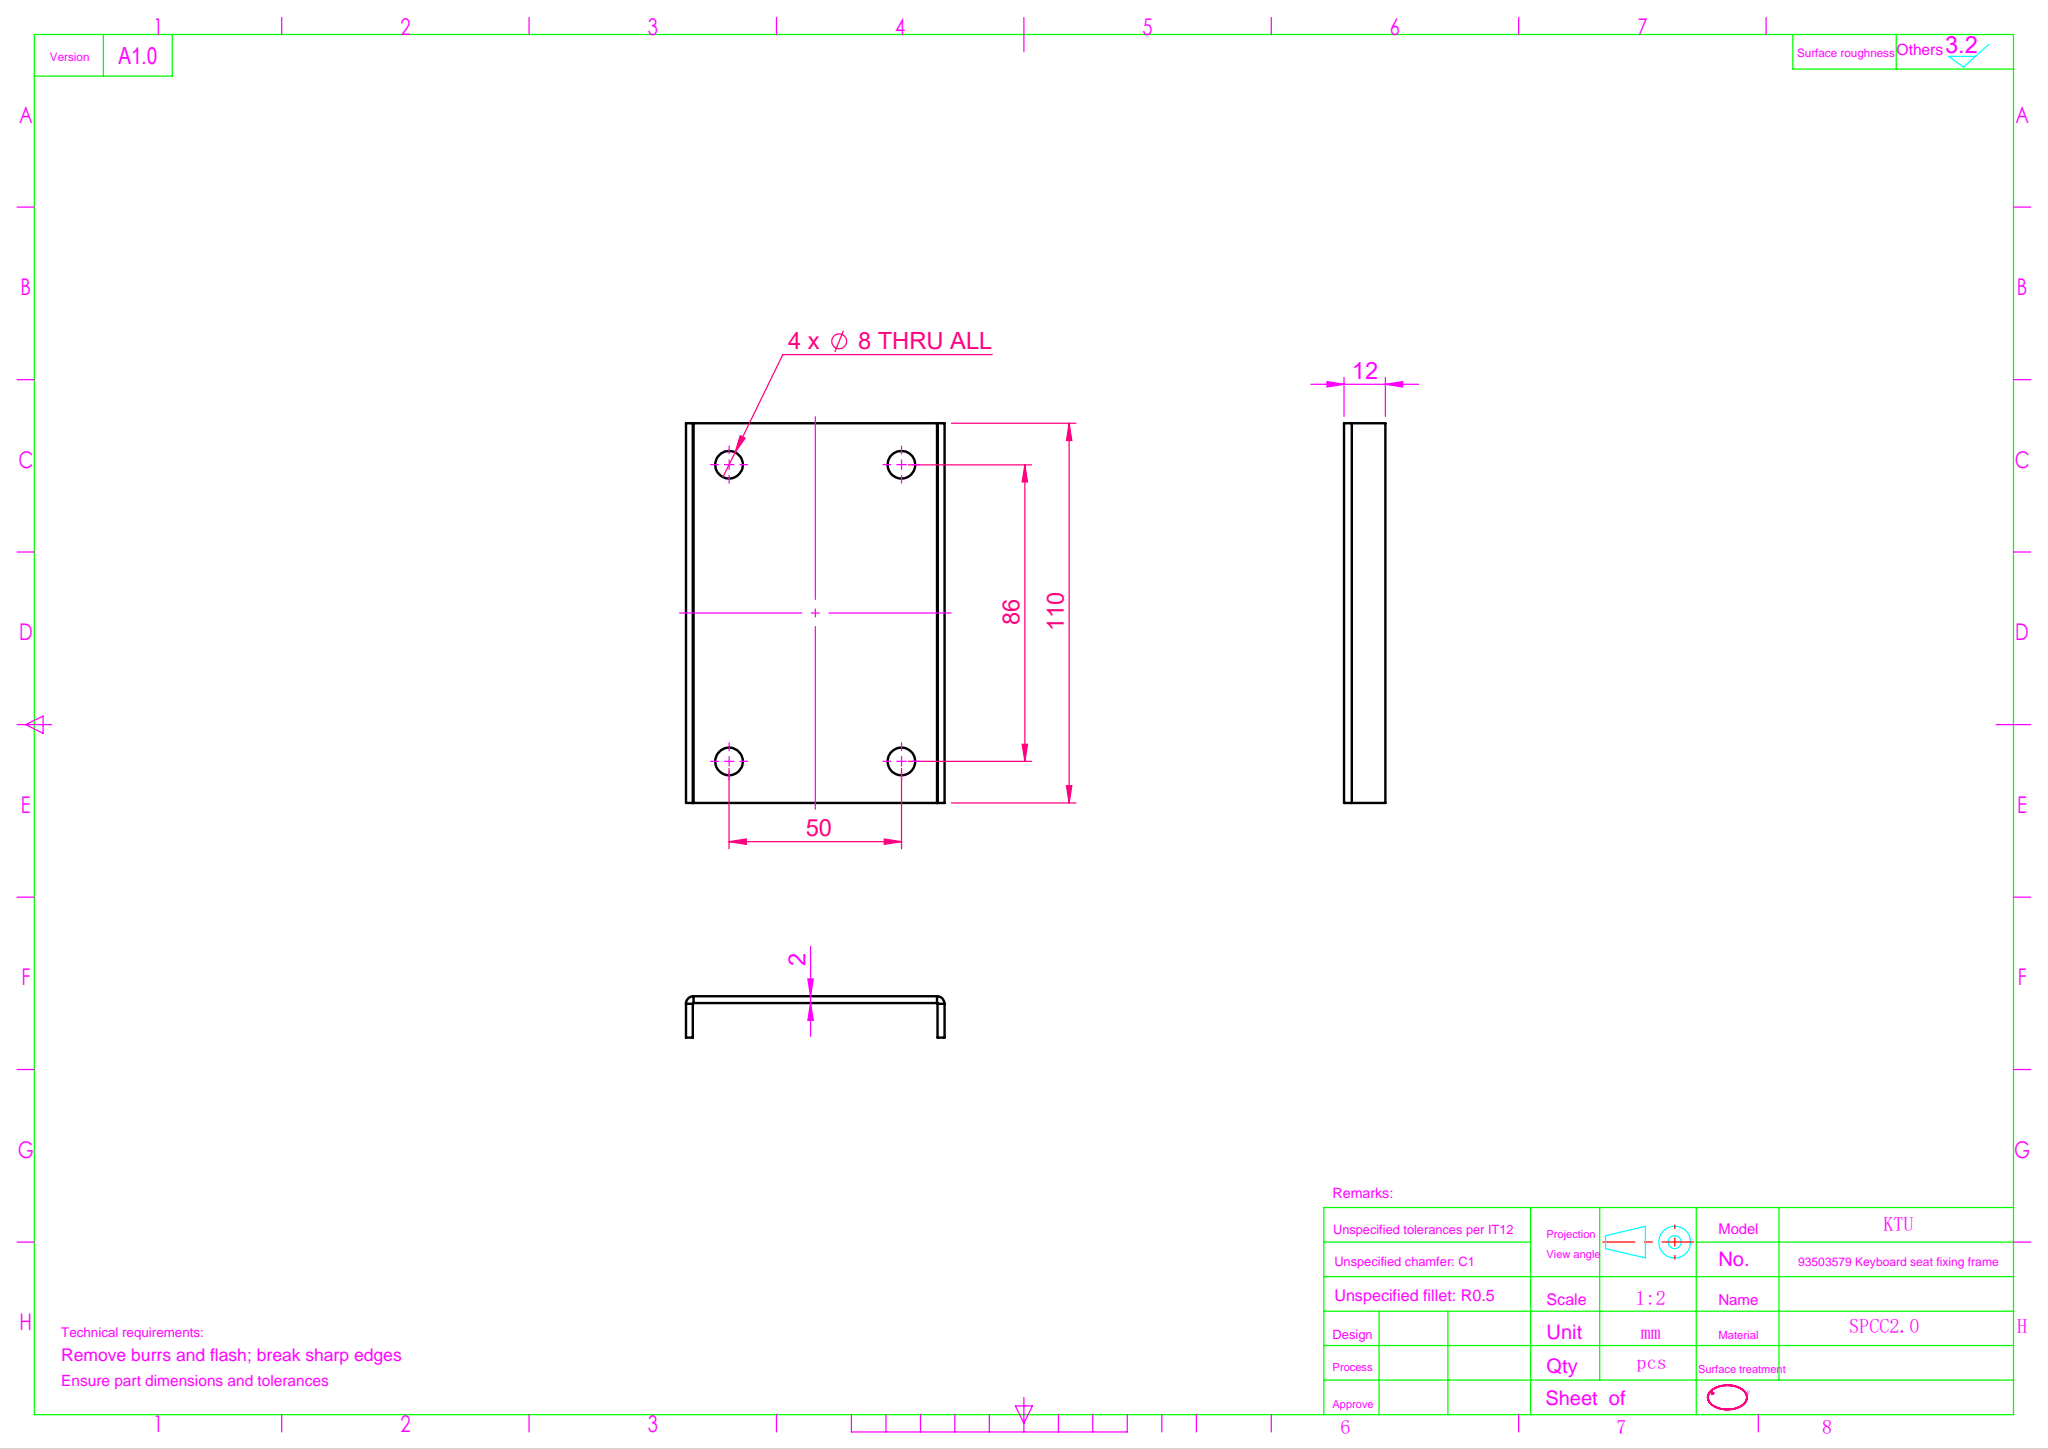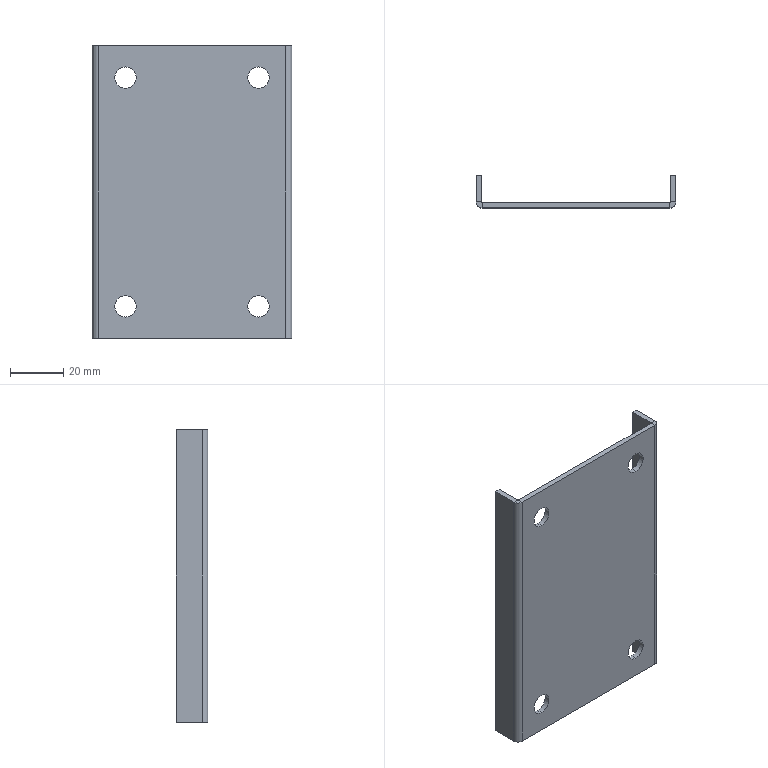Part | SolidWorks | features FlatPattern 1, HoleWzd 1, SMBaseFlange 1, SheetMetal 1 | 1 solid | 30 faces | box 75 x 12 x 110 mm | volume 20271 mm3 | plane 18 | cylinder 12 | commonest cylinder face diameters 8 x8 0.4 x2 4.4 x2
STEP:
#1=CARTESIAN_POINT('',(25.,2.,47.));
#2=VERTEX_POINT('',#1);
#3=CARTESIAN_POINT('',(25.,2.,39.));
#4=VERTEX_POINT('',#3);
#5=CARTESIAN_POINT('',(25.,2.,43.));
#6=DIRECTION('',(0.,-1.,0.));
#7=DIRECTION('',(0.,0.,-1.));
#8=AXIS2_PLACEMENT_3D('',#5,#6,#7);
#9=CIRCLE('',#8,4.);
#10=EDGE_CURVE('',#2,#4,#9,.T.);
#11=ORIENTED_EDGE('',*,*,#10,.F.);
#12=CARTESIAN_POINT('',(25.,0.,47.));
#13=VERTEX_POINT('',#12);
#14=CARTESIAN_POINT('',(25.,0.,47.));
#15=DIRECTION('',(0.,-1.,0.));
#16=VECTOR('',#15,1000.);
#17=LINE('',#14,#16);
#18=EDGE_CURVE('',#2,#13,#17,.T.);
#19=ORIENTED_EDGE('',*,*,#18,.T.);
#20=CARTESIAN_POINT('',(25.,0.,39.));
#21=VERTEX_POINT('',#20);
#22=CARTESIAN_POINT('',(25.,0.,43.));
#23=DIRECTION('',(0.,-1.,0.));
#24=DIRECTION('',(0.,0.,-1.));
#25=AXIS2_PLACEMENT_3D('',#22,#23,#24);
#26=CIRCLE('',#25,4.);
#27=EDGE_CURVE('',#13,#21,#26,.T.);
#28=ORIENTED_EDGE('',*,*,#27,.T.);
#29=CARTESIAN_POINT('',(25.,0.,39.));
#30=DIRECTION('',(0.,-1.,0.));
#31=VECTOR('',#30,1000.);
#32=LINE('',#29,#31);
#33=EDGE_CURVE('',#4,#21,#32,.T.);
#34=ORIENTED_EDGE('',*,*,#33,.F.);
#35=EDGE_LOOP('',(#11,#19,#28,#34));
#36=FACE_OUTER_BOUND('',#35,.T.);
#37=CARTESIAN_POINT('',(25.,0.,43.));
#38=DIRECTION('',(0.,-1.,0.));
#39=DIRECTION('',(0.,0.,-1.));
#40=AXIS2_PLACEMENT_3D('',#37,#38,#39);
#41=CYLINDRICAL_SURFACE('',#40,4.);
#42=ADVANCED_FACE('',(#36),#41,.F.);
#43=CARTESIAN_POINT('',(25.,2.,-39.));
#44=VERTEX_POINT('',#43);
#45=CARTESIAN_POINT('',(25.,2.,-47.));
#46=VERTEX_POINT('',#45);
#47=CARTESIAN_POINT('',(25.,2.,-43.));
#48=DIRECTION('',(0.,-1.,0.));
#49=DIRECTION('',(0.,0.,-1.));
#50=AXIS2_PLACEMENT_3D('',#47,#48,#49);
#51=CIRCLE('',#50,4.);
#52=EDGE_CURVE('',#44,#46,#51,.T.);
#53=ORIENTED_EDGE('',*,*,#52,.F.);
#54=CARTESIAN_POINT('',(25.,0.,-39.));
#55=VERTEX_POINT('',#54);
#56=CARTESIAN_POINT('',(25.,0.,-39.));
#57=DIRECTION('',(0.,-1.,0.));
#58=VECTOR('',#57,1000.);
#59=LINE('',#56,#58);
#60=EDGE_CURVE('',#44,#55,#59,.T.);
#61=ORIENTED_EDGE('',*,*,#60,.T.);
#62=CARTESIAN_POINT('',(25.,0.,-47.));
#63=VERTEX_POINT('',#62);
#64=CARTESIAN_POINT('',(25.,0.,-43.));
#65=DIRECTION('',(0.,-1.,0.));
#66=DIRECTION('',(0.,0.,-1.));
#67=AXIS2_PLACEMENT_3D('',#64,#65,#66);
#68=CIRCLE('',#67,4.);
#69=EDGE_CURVE('',#55,#63,#68,.T.);
#70=ORIENTED_EDGE('',*,*,#69,.T.);
#71=CARTESIAN_POINT('',(25.,0.,-47.));
#72=DIRECTION('',(0.,-1.,0.));
#73=VECTOR('',#72,1000.);
#74=LINE('',#71,#73);
#75=EDGE_CURVE('',#46,#63,#74,.T.);
#76=ORIENTED_EDGE('',*,*,#75,.F.);
#77=EDGE_LOOP('',(#53,#61,#70,#76));
#78=FACE_OUTER_BOUND('',#77,.T.);
#79=CARTESIAN_POINT('',(25.,0.,-43.));
#80=DIRECTION('',(0.,-1.,0.));
#81=DIRECTION('',(0.,0.,-1.));
#82=AXIS2_PLACEMENT_3D('',#79,#80,#81);
#83=CYLINDRICAL_SURFACE('',#82,4.);
#84=ADVANCED_FACE('',(#78),#83,.F.);
#85=CARTESIAN_POINT('',(-25.,2.,47.));
#86=VERTEX_POINT('',#85);
#87=CARTESIAN_POINT('',(-25.,2.,39.));
#88=VERTEX_POINT('',#87);
#89=CARTESIAN_POINT('',(-25.,2.,43.));
#90=DIRECTION('',(0.,-1.,0.));
#91=DIRECTION('',(0.,0.,-1.));
#92=AXIS2_PLACEMENT_3D('',#89,#90,#91);
#93=CIRCLE('',#92,4.);
#94=EDGE_CURVE('',#86,#88,#93,.T.);
#95=ORIENTED_EDGE('',*,*,#94,.F.);
#96=CARTESIAN_POINT('',(-25.,0.,47.));
#97=VERTEX_POINT('',#96);
#98=CARTESIAN_POINT('',(-25.,0.,47.));
#99=DIRECTION('',(0.,-1.,0.));
#100=VECTOR('',#99,1000.);
#101=LINE('',#98,#100);
#102=EDGE_CURVE('',#86,#97,#101,.T.);
#103=ORIENTED_EDGE('',*,*,#102,.T.);
#104=CARTESIAN_POINT('',(-25.,0.,39.));
#105=VERTEX_POINT('',#104);
#106=CARTESIAN_POINT('',(-25.,0.,43.));
#107=DIRECTION('',(0.,-1.,0.));
#108=DIRECTION('',(0.,0.,-1.));
#109=AXIS2_PLACEMENT_3D('',#106,#107,#108);
#110=CIRCLE('',#109,4.);
#111=EDGE_CURVE('',#97,#105,#110,.T.);
#112=ORIENTED_EDGE('',*,*,#111,.T.);
#113=CARTESIAN_POINT('',(-25.,0.,39.));
#114=DIRECTION('',(0.,-1.,0.));
#115=VECTOR('',#114,1000.);
#116=LINE('',#113,#115);
#117=EDGE_CURVE('',#88,#105,#116,.T.);
#118=ORIENTED_EDGE('',*,*,#117,.F.);
#119=EDGE_LOOP('',(#95,#103,#112,#118));
#120=FACE_OUTER_BOUND('',#119,.T.);
#121=CARTESIAN_POINT('',(-25.,0.,43.));
#122=DIRECTION('',(0.,-1.,0.));
#123=DIRECTION('',(0.,0.,-1.));
#124=AXIS2_PLACEMENT_3D('',#121,#122,#123);
#125=CYLINDRICAL_SURFACE('',#124,4.);
#126=ADVANCED_FACE('',(#120),#125,.F.);
#127=CARTESIAN_POINT('',(-25.,2.,-39.));
#128=VERTEX_POINT('',#127);
#129=CARTESIAN_POINT('',(-25.,2.,-47.));
#130=VERTEX_POINT('',#129);
#131=CARTESIAN_POINT('',(-25.,2.,-43.));
#132=DIRECTION('',(0.,-1.,0.));
#133=DIRECTION('',(0.,0.,-1.));
#134=AXIS2_PLACEMENT_3D('',#131,#132,#133);
#135=CIRCLE('',#134,4.);
#136=EDGE_CURVE('',#128,#130,#135,.T.);
#137=ORIENTED_EDGE('',*,*,#136,.F.);
#138=CARTESIAN_POINT('',(-25.,0.,-39.));
#139=VERTEX_POINT('',#138);
#140=CARTESIAN_POINT('',(-25.,0.,-39.));
#141=DIRECTION('',(0.,-1.,0.));
#142=VECTOR('',#141,1000.);
#143=LINE('',#140,#142);
#144=EDGE_CURVE('',#128,#139,#143,.T.);
#145=ORIENTED_EDGE('',*,*,#144,.T.);
#146=CARTESIAN_POINT('',(-25.,0.,-47.));
#147=VERTEX_POINT('',#146);
#148=CARTESIAN_POINT('',(-25.,0.,-43.));
#149=DIRECTION('',(0.,-1.,0.));
#150=DIRECTION('',(0.,0.,-1.));
#151=AXIS2_PLACEMENT_3D('',#148,#149,#150);
#152=CIRCLE('',#151,4.);
#153=EDGE_CURVE('',#139,#147,#152,.T.);
#154=ORIENTED_EDGE('',*,*,#153,.T.);
#155=CARTESIAN_POINT('',(-25.,0.,-47.));
#156=DIRECTION('',(0.,-1.,0.));
#157=VECTOR('',#156,1000.);
#158=LINE('',#155,#157);
#159=EDGE_CURVE('',#130,#147,#158,.T.);
#160=ORIENTED_EDGE('',*,*,#159,.F.);
#161=EDGE_LOOP('',(#137,#145,#154,#160));
#162=FACE_OUTER_BOUND('',#161,.T.);
#163=CARTESIAN_POINT('',(-25.,0.,-43.));
#164=DIRECTION('',(0.,-1.,0.));
#165=DIRECTION('',(0.,0.,-1.));
#166=AXIS2_PLACEMENT_3D('',#163,#164,#165);
#167=CYLINDRICAL_SURFACE('',#166,4.);
#168=ADVANCED_FACE('',(#162),#167,.F.);
#169=CARTESIAN_POINT('',(35.3,0.,55.));
#170=VERTEX_POINT('',#169);
#171=CARTESIAN_POINT('',(35.3,2.,55.));
#172=VERTEX_POINT('',#171);
#173=CARTESIAN_POINT('',(35.3,0.,55.));
#174=DIRECTION('',(0.,1.,0.));
#175=VECTOR('',#174,1000.);
#176=LINE('',#173,#175);
#177=EDGE_CURVE('',#170,#172,#176,.T.);
#178=ORIENTED_EDGE('',*,*,#177,.F.);
#179=CARTESIAN_POINT('',(37.5,2.2,55.));
#180=VERTEX_POINT('',#179);
#181=CARTESIAN_POINT('',(35.3,2.2,55.));
#182=DIRECTION('',(0.,0.,-1.));
#183=DIRECTION('',(1.,0.,0.));
#184=AXIS2_PLACEMENT_3D('',#181,#182,#183);
#185=CIRCLE('',#184,2.2);
#186=EDGE_CURVE('',#180,#170,#185,.T.);
#187=ORIENTED_EDGE('',*,*,#186,.F.);
#188=CARTESIAN_POINT('',(35.5,2.2,55.));
#189=VERTEX_POINT('',#188);
#190=CARTESIAN_POINT('',(35.5,2.2,55.));
#191=DIRECTION('',(1.,0.,0.));
#192=VECTOR('',#191,1000.);
#193=LINE('',#190,#192);
#194=EDGE_CURVE('',#189,#180,#193,.T.);
#195=ORIENTED_EDGE('',*,*,#194,.F.);
#196=CARTESIAN_POINT('',(35.3,2.2,55.));
#197=DIRECTION('',(0.,0.,-1.));
#198=DIRECTION('',(1.,0.,0.));
#199=AXIS2_PLACEMENT_3D('',#196,#197,#198);
#200=CIRCLE('',#199,0.2);
#201=EDGE_CURVE('',#189,#172,#200,.T.);
#202=ORIENTED_EDGE('',*,*,#201,.T.);
#203=EDGE_LOOP('',(#178,#187,#195,#202));
#204=FACE_OUTER_BOUND('',#203,.T.);
#205=CARTESIAN_POINT('',(35.3,0.,55.));
#206=DIRECTION('',(0.,0.,1.));
#207=DIRECTION('',(1.,0.,0.));
#208=AXIS2_PLACEMENT_3D('',#205,#206,#207);
#209=PLANE('',#208);
#210=ADVANCED_FACE('',(#204),#209,.T.);
#211=CARTESIAN_POINT('',(-35.3,0.,55.));
#212=VERTEX_POINT('',#211);
#213=CARTESIAN_POINT('',(-37.5,0.,55.));
#214=DIRECTION('',(-1.,0.,0.));
#215=VECTOR('',#214,1000.);
#216=LINE('',#213,#215);
#217=EDGE_CURVE('',#170,#212,#216,.T.);
#218=ORIENTED_EDGE('',*,*,#217,.F.);
#219=ORIENTED_EDGE('',*,*,#177,.T.);
#220=CARTESIAN_POINT('',(-35.3,2.,55.));
#221=VERTEX_POINT('',#220);
#222=CARTESIAN_POINT('',(-37.5,2.,55.));
#223=DIRECTION('',(-1.,0.,0.));
#224=VECTOR('',#223,1000.);
#225=LINE('',#222,#224);
#226=EDGE_CURVE('',#172,#221,#225,.T.);
#227=ORIENTED_EDGE('',*,*,#226,.T.);
#228=CARTESIAN_POINT('',(-35.3,2.,55.));
#229=DIRECTION('',(0.,-1.,0.));
#230=VECTOR('',#229,1000.);
#231=LINE('',#228,#230);
#232=EDGE_CURVE('',#221,#212,#231,.T.);
#233=ORIENTED_EDGE('',*,*,#232,.T.);
#234=EDGE_LOOP('',(#218,#219,#227,#233));
#235=FACE_OUTER_BOUND('',#234,.T.);
#236=CARTESIAN_POINT('',(35.5,2.2,55.));
#237=DIRECTION('',(0.,0.,1.));
#238=DIRECTION('',(1.,0.,0.));
#239=AXIS2_PLACEMENT_3D('',#236,#237,#238);
#240=PLANE('',#239);
#241=ADVANCED_FACE('',(#235),#240,.T.);
#242=CARTESIAN_POINT('',(37.5,2.2,-55.));
#243=VERTEX_POINT('',#242);
#244=CARTESIAN_POINT('',(35.5,2.2,-55.));
#245=VERTEX_POINT('',#244);
#246=CARTESIAN_POINT('',(37.5,2.2,-55.));
#247=DIRECTION('',(-1.,0.,0.));
#248=VECTOR('',#247,1000.);
#249=LINE('',#246,#248);
#250=EDGE_CURVE('',#243,#245,#249,.T.);
#251=ORIENTED_EDGE('',*,*,#250,.F.);
#252=CARTESIAN_POINT('',(35.3,0.,-55.));
#253=VERTEX_POINT('',#252);
#254=CARTESIAN_POINT('',(35.3,2.2,-55.));
#255=DIRECTION('',(0.,0.,-1.));
#256=DIRECTION('',(1.,0.,0.));
#257=AXIS2_PLACEMENT_3D('',#254,#255,#256);
#258=CIRCLE('',#257,2.2);
#259=EDGE_CURVE('',#243,#253,#258,.T.);
#260=ORIENTED_EDGE('',*,*,#259,.T.);
#261=CARTESIAN_POINT('',(35.3,2.,-55.));
#262=VERTEX_POINT('',#261);
#263=CARTESIAN_POINT('',(35.3,2.,-55.));
#264=DIRECTION('',(0.,-1.,0.));
#265=VECTOR('',#264,1000.);
#266=LINE('',#263,#265);
#267=EDGE_CURVE('',#262,#253,#266,.T.);
#268=ORIENTED_EDGE('',*,*,#267,.F.);
#269=CARTESIAN_POINT('',(35.3,2.2,-55.));
#270=DIRECTION('',(0.,0.,-1.));
#271=DIRECTION('',(1.,0.,0.));
#272=AXIS2_PLACEMENT_3D('',#269,#270,#271);
#273=CIRCLE('',#272,0.2);
#274=EDGE_CURVE('',#245,#262,#273,.T.);
#275=ORIENTED_EDGE('',*,*,#274,.F.);
#276=EDGE_LOOP('',(#251,#260,#268,#275));
#277=FACE_OUTER_BOUND('',#276,.T.);
#278=CARTESIAN_POINT('',(37.5,2.2,-55.));
#279=DIRECTION('',(0.,0.,-1.));
#280=DIRECTION('',(-1.,0.,0.));
#281=AXIS2_PLACEMENT_3D('',#278,#279,#280);
#282=PLANE('',#281);
#283=ADVANCED_FACE('',(#277),#282,.T.);
#284=CARTESIAN_POINT('',(37.5,12.,-55.));
#285=VERTEX_POINT('',#284);
#286=CARTESIAN_POINT('',(37.5,0.,-55.));
#287=DIRECTION('',(0.,-1.,0.));
#288=VECTOR('',#287,1000.);
#289=LINE('',#286,#288);
#290=EDGE_CURVE('',#285,#243,#289,.T.);
#291=ORIENTED_EDGE('',*,*,#290,.T.);
#292=ORIENTED_EDGE('',*,*,#250,.T.);
#293=CARTESIAN_POINT('',(35.5,12.,-55.));
#294=VERTEX_POINT('',#293);
#295=CARTESIAN_POINT('',(35.5,0.,-55.));
#296=DIRECTION('',(0.,-1.,0.));
#297=VECTOR('',#296,1000.);
#298=LINE('',#295,#297);
#299=EDGE_CURVE('',#294,#245,#298,.T.);
#300=ORIENTED_EDGE('',*,*,#299,.F.);
#301=CARTESIAN_POINT('',(35.5,12.,-55.));
#302=DIRECTION('',(1.,0.,0.));
#303=VECTOR('',#302,1000.);
#304=LINE('',#301,#303);
#305=EDGE_CURVE('',#294,#285,#304,.T.);
#306=ORIENTED_EDGE('',*,*,#305,.T.);
#307=EDGE_LOOP('',(#291,#292,#300,#306));
#308=FACE_OUTER_BOUND('',#307,.T.);
#309=CARTESIAN_POINT('',(35.3,2.,-55.));
#310=DIRECTION('',(0.,0.,-1.));
#311=DIRECTION('',(-1.,0.,0.));
#312=AXIS2_PLACEMENT_3D('',#309,#310,#311);
#313=PLANE('',#312);
#314=ADVANCED_FACE('',(#308),#313,.T.);
#315=CARTESIAN_POINT('',(-37.5,2.2,55.));
#316=VERTEX_POINT('',#315);
#317=CARTESIAN_POINT('',(-35.5,2.2,55.));
#318=VERTEX_POINT('',#317);
#319=CARTESIAN_POINT('',(-37.5,2.2,55.));
#320=DIRECTION('',(1.,0.,0.));
#321=VECTOR('',#320,1000.);
#322=LINE('',#319,#321);
#323=EDGE_CURVE('',#316,#318,#322,.T.);
#324=ORIENTED_EDGE('',*,*,#323,.F.);
#325=CARTESIAN_POINT('',(-35.3,2.2,55.));
#326=DIRECTION('',(0.,0.,-1.));
#327=DIRECTION('',(1.,0.,0.));
#328=AXIS2_PLACEMENT_3D('',#325,#326,#327);
#329=CIRCLE('',#328,2.2);
#330=EDGE_CURVE('',#212,#316,#329,.T.);
#331=ORIENTED_EDGE('',*,*,#330,.F.);
#332=ORIENTED_EDGE('',*,*,#232,.F.);
#333=CARTESIAN_POINT('',(-35.3,2.2,55.));
#334=DIRECTION('',(0.,0.,-1.));
#335=DIRECTION('',(1.,0.,0.));
#336=AXIS2_PLACEMENT_3D('',#333,#334,#335);
#337=CIRCLE('',#336,0.2);
#338=EDGE_CURVE('',#221,#318,#337,.T.);
#339=ORIENTED_EDGE('',*,*,#338,.T.);
#340=EDGE_LOOP('',(#324,#331,#332,#339));
#341=FACE_OUTER_BOUND('',#340,.T.);
#342=CARTESIAN_POINT('',(-37.5,2.2,55.));
#343=DIRECTION('',(0.,0.,1.));
#344=DIRECTION('',(1.,0.,0.));
#345=AXIS2_PLACEMENT_3D('',#342,#343,#344);
#346=PLANE('',#345);
#347=ADVANCED_FACE('',(#341),#346,.T.);
#348=CARTESIAN_POINT('',(-37.5,12.,55.));
#349=VERTEX_POINT('',#348);
#350=CARTESIAN_POINT('',(-37.5,0.,55.));
#351=DIRECTION('',(0.,1.,0.));
#352=VECTOR('',#351,1000.);
#353=LINE('',#350,#352);
#354=EDGE_CURVE('',#316,#349,#353,.T.);
#355=ORIENTED_EDGE('',*,*,#354,.F.);
#356=ORIENTED_EDGE('',*,*,#323,.T.);
#357=CARTESIAN_POINT('',(-35.5,12.,55.));
#358=VERTEX_POINT('',#357);
#359=CARTESIAN_POINT('',(-35.5,0.,55.));
#360=DIRECTION('',(0.,1.,0.));
#361=VECTOR('',#360,1000.);
#362=LINE('',#359,#361);
#363=EDGE_CURVE('',#318,#358,#362,.T.);
#364=ORIENTED_EDGE('',*,*,#363,.T.);
#365=CARTESIAN_POINT('',(-37.5,12.,55.));
#366=DIRECTION('',(1.,0.,0.));
#367=VECTOR('',#366,1000.);
#368=LINE('',#365,#367);
#369=EDGE_CURVE('',#349,#358,#368,.T.);
#370=ORIENTED_EDGE('',*,*,#369,.F.);
#371=EDGE_LOOP('',(#355,#356,#364,#370));
#372=FACE_OUTER_BOUND('',#371,.T.);
#373=CARTESIAN_POINT('',(-35.3,2.,55.));
#374=DIRECTION('',(0.,0.,1.));
#375=DIRECTION('',(1.,0.,0.));
#376=AXIS2_PLACEMENT_3D('',#373,#374,#375);
#377=PLANE('',#376);
#378=ADVANCED_FACE('',(#372),#377,.T.);
#379=CARTESIAN_POINT('',(-35.3,0.,-55.));
#380=VERTEX_POINT('',#379);
#381=CARTESIAN_POINT('',(-35.3,2.,-55.));
#382=VERTEX_POINT('',#381);
#383=CARTESIAN_POINT('',(-35.3,0.,-55.));
#384=DIRECTION('',(0.,1.,0.));
#385=VECTOR('',#384,1000.);
#386=LINE('',#383,#385);
#387=EDGE_CURVE('',#380,#382,#386,.T.);
#388=ORIENTED_EDGE('',*,*,#387,.F.);
#389=CARTESIAN_POINT('',(-37.5,2.2,-55.));
#390=VERTEX_POINT('',#389);
#391=CARTESIAN_POINT('',(-35.3,2.2,-55.));
#392=DIRECTION('',(0.,0.,-1.));
#393=DIRECTION('',(1.,0.,0.));
#394=AXIS2_PLACEMENT_3D('',#391,#392,#393);
#395=CIRCLE('',#394,2.2);
#396=EDGE_CURVE('',#380,#390,#395,.T.);
#397=ORIENTED_EDGE('',*,*,#396,.T.);
#398=CARTESIAN_POINT('',(-35.5,2.2,-55.));
#399=VERTEX_POINT('',#398);
#400=CARTESIAN_POINT('',(-35.5,2.2,-55.));
#401=DIRECTION('',(-1.,0.,0.));
#402=VECTOR('',#401,1000.);
#403=LINE('',#400,#402);
#404=EDGE_CURVE('',#399,#390,#403,.T.);
#405=ORIENTED_EDGE('',*,*,#404,.F.);
#406=CARTESIAN_POINT('',(-35.3,2.2,-55.));
#407=DIRECTION('',(0.,0.,-1.));
#408=DIRECTION('',(1.,0.,0.));
#409=AXIS2_PLACEMENT_3D('',#406,#407,#408);
#410=CIRCLE('',#409,0.2);
#411=EDGE_CURVE('',#382,#399,#410,.T.);
#412=ORIENTED_EDGE('',*,*,#411,.F.);
#413=EDGE_LOOP('',(#388,#397,#405,#412));
#414=FACE_OUTER_BOUND('',#413,.T.);
#415=CARTESIAN_POINT('',(-35.3,0.,-55.));
#416=DIRECTION('',(0.,0.,-1.));
#417=DIRECTION('',(-1.,0.,0.));
#418=AXIS2_PLACEMENT_3D('',#415,#416,#417);
#419=PLANE('',#418);
#420=ADVANCED_FACE('',(#414),#419,.T.);
#421=CARTESIAN_POINT('',(-37.5,0.,-55.));
#422=DIRECTION('',(-1.,0.,0.));
#423=VECTOR('',#422,1000.);
#424=LINE('',#421,#423);
#425=EDGE_CURVE('',#253,#380,#424,.T.);
#426=ORIENTED_EDGE('',*,*,#425,.T.);
#427=ORIENTED_EDGE('',*,*,#387,.T.);
#428=CARTESIAN_POINT('',(-37.5,2.,-55.));
#429=DIRECTION('',(-1.,0.,0.));
#430=VECTOR('',#429,1000.);
#431=LINE('',#428,#430);
#432=EDGE_CURVE('',#262,#382,#431,.T.);
#433=ORIENTED_EDGE('',*,*,#432,.F.);
#434=ORIENTED_EDGE('',*,*,#267,.T.);
#435=EDGE_LOOP('',(#426,#427,#433,#434));
#436=FACE_OUTER_BOUND('',#435,.T.);
#437=CARTESIAN_POINT('',(-35.5,2.2,-55.));
#438=DIRECTION('',(0.,0.,-1.));
#439=DIRECTION('',(-1.,0.,0.));
#440=AXIS2_PLACEMENT_3D('',#437,#438,#439);
#441=PLANE('',#440);
#442=ADVANCED_FACE('',(#436),#441,.T.);
#443=CARTESIAN_POINT('',(-35.5,12.,-55.));
#444=VERTEX_POINT('',#443);
#445=CARTESIAN_POINT('',(-35.5,0.,-55.));
#446=DIRECTION('',(0.,1.,0.));
#447=VECTOR('',#446,1000.);
#448=LINE('',#445,#447);
#449=EDGE_CURVE('',#399,#444,#448,.T.);
#450=ORIENTED_EDGE('',*,*,#449,.T.);
#451=CARTESIAN_POINT('',(-35.5,12.,55.));
#452=DIRECTION('',(0.,0.,-1.));
#453=VECTOR('',#452,1000.);
#454=LINE('',#451,#453);
#455=EDGE_CURVE('',#358,#444,#454,.T.);
#456=ORIENTED_EDGE('',*,*,#455,.F.);
#457=ORIENTED_EDGE('',*,*,#363,.F.);
#458=CARTESIAN_POINT('',(-35.5,2.2,55.));
#459=DIRECTION('',(0.,0.,-1.));
#460=VECTOR('',#459,1000.);
#461=LINE('',#458,#460);
#462=EDGE_CURVE('',#318,#399,#461,.T.);
#463=ORIENTED_EDGE('',*,*,#462,.T.);
#464=EDGE_LOOP('',(#450,#456,#457,#463));
#465=FACE_OUTER_BOUND('',#464,.T.);
#466=CARTESIAN_POINT('',(-35.5,0.,55.));
#467=DIRECTION('',(-1.,0.,0.));
#468=DIRECTION('',(0.,0.,1.));
#469=AXIS2_PLACEMENT_3D('',#466,#467,#468);
#470=PLANE('',#469);
#471=ADVANCED_FACE('',(#465),#470,.F.);
#472=CARTESIAN_POINT('',(-37.5,12.,-55.));
#473=VERTEX_POINT('',#472);
#474=CARTESIAN_POINT('',(-37.5,12.,-55.));
#475=DIRECTION('',(1.,0.,0.));
#476=VECTOR('',#475,1000.);
#477=LINE('',#474,#476);
#478=EDGE_CURVE('',#473,#444,#477,.T.);
#479=ORIENTED_EDGE('',*,*,#478,.F.);
#480=CARTESIAN_POINT('',(-37.5,12.,55.));
#481=DIRECTION('',(0.,0.,-1.));
#482=VECTOR('',#481,1000.);
#483=LINE('',#480,#482);
#484=EDGE_CURVE('',#349,#473,#483,.T.);
#485=ORIENTED_EDGE('',*,*,#484,.F.);
#486=ORIENTED_EDGE('',*,*,#369,.T.);
#487=ORIENTED_EDGE('',*,*,#455,.T.);
#488=EDGE_LOOP('',(#479,#485,#486,#487));
#489=FACE_OUTER_BOUND('',#488,.T.);
#490=CARTESIAN_POINT('',(-37.5,12.,55.));
#491=DIRECTION('',(0.,1.,0.));
#492=DIRECTION('',(0.,0.,1.));
#493=AXIS2_PLACEMENT_3D('',#490,#491,#492);
#494=PLANE('',#493);
#495=ADVANCED_FACE('',(#489),#494,.T.);
#496=CARTESIAN_POINT('',(-37.5,0.,-55.));
#497=DIRECTION('',(0.,1.,0.));
#498=VECTOR('',#497,1000.);
#499=LINE('',#496,#498);
#500=EDGE_CURVE('',#390,#473,#499,.T.);
#501=ORIENTED_EDGE('',*,*,#500,.F.);
#502=CARTESIAN_POINT('',(-37.5,2.2,55.));
#503=DIRECTION('',(0.,0.,-1.));
#504=VECTOR('',#503,1000.);
#505=LINE('',#502,#504);
#506=EDGE_CURVE('',#316,#390,#505,.T.);
#507=ORIENTED_EDGE('',*,*,#506,.F.);
#508=ORIENTED_EDGE('',*,*,#354,.T.);
#509=ORIENTED_EDGE('',*,*,#484,.T.);
#510=EDGE_LOOP('',(#501,#507,#508,#509));
#511=FACE_OUTER_BOUND('',#510,.T.);
#512=CARTESIAN_POINT('',(-37.5,0.,55.));
#513=DIRECTION('',(-1.,0.,0.));
#514=DIRECTION('',(0.,0.,1.));
#515=AXIS2_PLACEMENT_3D('',#512,#513,#514);
#516=PLANE('',#515);
#517=ADVANCED_FACE('',(#511),#516,.T.);
#518=ORIENTED_EDGE('',*,*,#396,.F.);
#519=CARTESIAN_POINT('',(-35.3,0.,55.));
#520=DIRECTION('',(0.,0.,-1.));
#521=VECTOR('',#520,1000.);
#522=LINE('',#519,#521);
#523=EDGE_CURVE('',#212,#380,#522,.T.);
#524=ORIENTED_EDGE('',*,*,#523,.F.);
#525=ORIENTED_EDGE('',*,*,#330,.T.);
#526=ORIENTED_EDGE('',*,*,#506,.T.);
#527=EDGE_LOOP('',(#518,#524,#525,#526));
#528=FACE_OUTER_BOUND('',#527,.T.);
#529=CARTESIAN_POINT('',(-35.3,2.2,55.));
#530=DIRECTION('',(0.,0.,-1.));
#531=DIRECTION('',(-1.,0.,0.));
#532=AXIS2_PLACEMENT_3D('',#529,#530,#531);
#533=CYLINDRICAL_SURFACE('',#532,2.2);
#534=ADVANCED_FACE('',(#528),#533,.T.);
#535=CARTESIAN_POINT('',(25.,0.,43.));
#536=DIRECTION('',(0.,-1.,0.));
#537=DIRECTION('',(0.,0.,-1.));
#538=AXIS2_PLACEMENT_3D('',#535,#536,#537);
#539=CIRCLE('',#538,4.);
#540=EDGE_CURVE('',#21,#13,#539,.T.);
#541=ORIENTED_EDGE('',*,*,#540,.F.);
#542=ORIENTED_EDGE('',*,*,#27,.F.);
#543=EDGE_LOOP('',(#541,#542));
#544=FACE_BOUND('',#543,.T.);
#545=CARTESIAN_POINT('',(25.,0.,-43.));
#546=DIRECTION('',(0.,-1.,0.));
#547=DIRECTION('',(0.,0.,-1.));
#548=AXIS2_PLACEMENT_3D('',#545,#546,#547);
#549=CIRCLE('',#548,4.);
#550=EDGE_CURVE('',#63,#55,#549,.T.);
#551=ORIENTED_EDGE('',*,*,#550,.F.);
#552=ORIENTED_EDGE('',*,*,#69,.F.);
#553=EDGE_LOOP('',(#551,#552));
#554=FACE_BOUND('',#553,.T.);
#555=CARTESIAN_POINT('',(-25.,0.,43.));
#556=DIRECTION('',(0.,-1.,0.));
#557=DIRECTION('',(0.,0.,-1.));
#558=AXIS2_PLACEMENT_3D('',#555,#556,#557);
#559=CIRCLE('',#558,4.);
#560=EDGE_CURVE('',#105,#97,#559,.T.);
#561=ORIENTED_EDGE('',*,*,#560,.F.);
#562=ORIENTED_EDGE('',*,*,#111,.F.);
#563=EDGE_LOOP('',(#561,#562));
#564=FACE_BOUND('',#563,.T.);
#565=CARTESIAN_POINT('',(-25.,0.,-43.));
#566=DIRECTION('',(0.,-1.,0.));
#567=DIRECTION('',(0.,0.,-1.));
#568=AXIS2_PLACEMENT_3D('',#565,#566,#567);
#569=CIRCLE('',#568,4.);
#570=EDGE_CURVE('',#147,#139,#569,.T.);
#571=ORIENTED_EDGE('',*,*,#570,.F.);
#572=ORIENTED_EDGE('',*,*,#153,.F.);
#573=EDGE_LOOP('',(#571,#572));
#574=FACE_BOUND('',#573,.T.);
#575=ORIENTED_EDGE('',*,*,#425,.F.);
#576=CARTESIAN_POINT('',(35.3,0.,55.));
#577=DIRECTION('',(0.,0.,-1.));
#578=VECTOR('',#577,1000.);
#579=LINE('',#576,#578);
#580=EDGE_CURVE('',#170,#253,#579,.T.);
#581=ORIENTED_EDGE('',*,*,#580,.F.);
#582=ORIENTED_EDGE('',*,*,#217,.T.);
#583=ORIENTED_EDGE('',*,*,#523,.T.);
#584=EDGE_LOOP('',(#575,#581,#582,#583));
#585=FACE_OUTER_BOUND('',#584,.T.);
#586=CARTESIAN_POINT('',(-37.5,0.,55.));
#587=DIRECTION('',(0.,-1.,0.));
#588=DIRECTION('',(0.,0.,-1.));
#589=AXIS2_PLACEMENT_3D('',#586,#587,#588);
#590=PLANE('',#589);
#591=ADVANCED_FACE('',(#544,#554,#564,#574,#585),#590,.T.);
#592=ORIENTED_EDGE('',*,*,#259,.F.);
#593=CARTESIAN_POINT('',(37.5,2.2,55.));
#594=DIRECTION('',(0.,0.,-1.));
#595=VECTOR('',#594,1000.);
#596=LINE('',#593,#595);
#597=EDGE_CURVE('',#180,#243,#596,.T.);
#598=ORIENTED_EDGE('',*,*,#597,.F.);
#599=ORIENTED_EDGE('',*,*,#186,.T.);
#600=ORIENTED_EDGE('',*,*,#580,.T.);
#601=EDGE_LOOP('',(#592,#598,#599,#600));
#602=FACE_OUTER_BOUND('',#601,.T.);
#603=CARTESIAN_POINT('',(35.3,2.2,55.));
#604=DIRECTION('',(0.,0.,-1.));
#605=DIRECTION('',(-1.,0.,0.));
#606=AXIS2_PLACEMENT_3D('',#603,#604,#605);
#607=CYLINDRICAL_SURFACE('',#606,2.2);
#608=ADVANCED_FACE('',(#602),#607,.T.);
#609=ORIENTED_EDGE('',*,*,#290,.F.);
#610=CARTESIAN_POINT('',(37.5,12.,55.));
#611=VERTEX_POINT('',#610);
#612=CARTESIAN_POINT('',(37.5,12.,55.));
#613=DIRECTION('',(0.,0.,-1.));
#614=VECTOR('',#613,1000.);
#615=LINE('',#612,#614);
#616=EDGE_CURVE('',#611,#285,#615,.T.);
#617=ORIENTED_EDGE('',*,*,#616,.F.);
#618=CARTESIAN_POINT('',(37.5,0.,55.));
#619=DIRECTION('',(0.,-1.,0.));
#620=VECTOR('',#619,1000.);
#621=LINE('',#618,#620);
#622=EDGE_CURVE('',#611,#180,#621,.T.);
#623=ORIENTED_EDGE('',*,*,#622,.T.);
#624=ORIENTED_EDGE('',*,*,#597,.T.);
#625=EDGE_LOOP('',(#609,#617,#623,#624));
#626=FACE_OUTER_BOUND('',#625,.T.);
#627=CARTESIAN_POINT('',(37.5,0.,55.));
#628=DIRECTION('',(1.,0.,0.));
#629=DIRECTION('',(0.,0.,-1.));
#630=AXIS2_PLACEMENT_3D('',#627,#628,#629);
#631=PLANE('',#630);
#632=ADVANCED_FACE('',(#626),#631,.T.);
#633=ORIENTED_EDGE('',*,*,#305,.F.);
#634=CARTESIAN_POINT('',(35.5,12.,55.));
#635=VERTEX_POINT('',#634);
#636=CARTESIAN_POINT('',(35.5,12.,55.));
#637=DIRECTION('',(0.,0.,-1.));
#638=VECTOR('',#637,1000.);
#639=LINE('',#636,#638);
#640=EDGE_CURVE('',#635,#294,#639,.T.);
#641=ORIENTED_EDGE('',*,*,#640,.F.);
#642=CARTESIAN_POINT('',(35.5,12.,55.));
#643=DIRECTION('',(1.,0.,0.));
#644=VECTOR('',#643,1000.);
#645=LINE('',#642,#644);
#646=EDGE_CURVE('',#635,#611,#645,.T.);
#647=ORIENTED_EDGE('',*,*,#646,.T.);
#648=ORIENTED_EDGE('',*,*,#616,.T.);
#649=EDGE_LOOP('',(#633,#641,#647,#648));
#650=FACE_OUTER_BOUND('',#649,.T.);
#651=CARTESIAN_POINT('',(35.5,12.,55.));
#652=DIRECTION('',(0.,1.,0.));
#653=DIRECTION('',(0.,0.,1.));
#654=AXIS2_PLACEMENT_3D('',#651,#652,#653);
#655=PLANE('',#654);
#656=ADVANCED_FACE('',(#650),#655,.T.);
#657=ORIENTED_EDGE('',*,*,#299,.T.);
#658=CARTESIAN_POINT('',(35.5,2.2,55.));
#659=DIRECTION('',(0.,0.,-1.));
#660=VECTOR('',#659,1000.);
#661=LINE('',#658,#660);
#662=EDGE_CURVE('',#189,#245,#661,.T.);
#663=ORIENTED_EDGE('',*,*,#662,.F.);
#664=CARTESIAN_POINT('',(35.5,0.,55.));
#665=DIRECTION('',(0.,-1.,0.));
#666=VECTOR('',#665,1000.);
#667=LINE('',#664,#666);
#668=EDGE_CURVE('',#635,#189,#667,.T.);
#669=ORIENTED_EDGE('',*,*,#668,.F.);
#670=ORIENTED_EDGE('',*,*,#640,.T.);
#671=EDGE_LOOP('',(#657,#663,#669,#670));
#672=FACE_OUTER_BOUND('',#671,.T.);
#673=CARTESIAN_POINT('',(35.5,0.,55.));
#674=DIRECTION('',(1.,0.,0.));
#675=DIRECTION('',(0.,0.,-1.));
#676=AXIS2_PLACEMENT_3D('',#673,#674,#675);
#677=PLANE('',#676);
#678=ADVANCED_FACE('',(#672),#677,.F.);
#679=ORIENTED_EDGE('',*,*,#274,.T.);
#680=CARTESIAN_POINT('',(35.3,2.,55.));
#681=DIRECTION('',(0.,0.,-1.));
#682=VECTOR('',#681,1000.);
#683=LINE('',#680,#682);
#684=EDGE_CURVE('',#172,#262,#683,.T.);
#685=ORIENTED_EDGE('',*,*,#684,.F.);
#686=ORIENTED_EDGE('',*,*,#201,.F.);
#687=ORIENTED_EDGE('',*,*,#662,.T.);
#688=EDGE_LOOP('',(#679,#685,#686,#687));
#689=FACE_OUTER_BOUND('',#688,.T.);
#690=CARTESIAN_POINT('',(35.3,2.2,55.));
#691=DIRECTION('',(0.,0.,-1.));
#692=DIRECTION('',(-1.,0.,0.));
#693=AXIS2_PLACEMENT_3D('',#690,#691,#692);
#694=CYLINDRICAL_SURFACE('',#693,0.2);
#695=ADVANCED_FACE('',(#689),#694,.F.);
#696=CARTESIAN_POINT('',(25.,2.,43.));
#697=DIRECTION('',(0.,-1.,0.));
#698=DIRECTION('',(0.,0.,-1.));
#699=AXIS2_PLACEMENT_3D('',#696,#697,#698);
#700=CIRCLE('',#699,4.);
#701=EDGE_CURVE('',#4,#2,#700,.T.);
#702=ORIENTED_EDGE('',*,*,#701,.T.);
#703=ORIENTED_EDGE('',*,*,#10,.T.);
#704=EDGE_LOOP('',(#702,#703));
#705=FACE_BOUND('',#704,.T.);
#706=CARTESIAN_POINT('',(25.,2.,-43.));
#707=DIRECTION('',(0.,-1.,0.));
#708=DIRECTION('',(0.,0.,-1.));
#709=AXIS2_PLACEMENT_3D('',#706,#707,#708);
#710=CIRCLE('',#709,4.);
#711=EDGE_CURVE('',#46,#44,#710,.T.);
#712=ORIENTED_EDGE('',*,*,#711,.T.);
#713=ORIENTED_EDGE('',*,*,#52,.T.);
#714=EDGE_LOOP('',(#712,#713));
#715=FACE_BOUND('',#714,.T.);
#716=CARTESIAN_POINT('',(-25.,2.,43.));
#717=DIRECTION('',(0.,-1.,0.));
#718=DIRECTION('',(0.,0.,-1.));
#719=AXIS2_PLACEMENT_3D('',#716,#717,#718);
#720=CIRCLE('',#719,4.);
#721=EDGE_CURVE('',#88,#86,#720,.T.);
#722=ORIENTED_EDGE('',*,*,#721,.T.);
#723=ORIENTED_EDGE('',*,*,#94,.T.);
#724=EDGE_LOOP('',(#722,#723));
#725=FACE_BOUND('',#724,.T.);
#726=CARTESIAN_POINT('',(-25.,2.,-43.));
#727=DIRECTION('',(0.,-1.,0.));
#728=DIRECTION('',(0.,0.,-1.));
#729=AXIS2_PLACEMENT_3D('',#726,#727,#728);
#730=CIRCLE('',#729,4.);
#731=EDGE_CURVE('',#130,#128,#730,.T.);
#732=ORIENTED_EDGE('',*,*,#731,.T.);
#733=ORIENTED_EDGE('',*,*,#136,.T.);
#734=EDGE_LOOP('',(#732,#733));
#735=FACE_BOUND('',#734,.T.);
#736=ORIENTED_EDGE('',*,*,#432,.T.);
#737=CARTESIAN_POINT('',(-35.3,2.,55.));
#738=DIRECTION('',(0.,0.,-1.));
#739=VECTOR('',#738,1000.);
#740=LINE('',#737,#739);
#741=EDGE_CURVE('',#221,#382,#740,.T.);
#742=ORIENTED_EDGE('',*,*,#741,.F.);
#743=ORIENTED_EDGE('',*,*,#226,.F.);
#744=ORIENTED_EDGE('',*,*,#684,.T.);
#745=EDGE_LOOP('',(#736,#742,#743,#744));
#746=FACE_OUTER_BOUND('',#745,.T.);
#747=CARTESIAN_POINT('',(-37.5,2.,55.));
#748=DIRECTION('',(0.,-1.,0.));
#749=DIRECTION('',(0.,0.,-1.));
#750=AXIS2_PLACEMENT_3D('',#747,#748,#749);
#751=PLANE('',#750);
#752=ADVANCED_FACE('',(#705,#715,#725,#735,#746),#751,.F.);
#753=ORIENTED_EDGE('',*,*,#411,.T.);
#754=ORIENTED_EDGE('',*,*,#462,.F.);
#755=ORIENTED_EDGE('',*,*,#338,.F.);
#756=ORIENTED_EDGE('',*,*,#741,.T.);
#757=EDGE_LOOP('',(#753,#754,#755,#756));
#758=FACE_OUTER_BOUND('',#757,.T.);
#759=CARTESIAN_POINT('',(-35.3,2.2,55.));
#760=DIRECTION('',(0.,0.,-1.));
#761=DIRECTION('',(-1.,0.,0.));
#762=AXIS2_PLACEMENT_3D('',#759,#760,#761);
#763=CYLINDRICAL_SURFACE('',#762,0.2);
#764=ADVANCED_FACE('',(#758),#763,.F.);
#765=ORIENTED_EDGE('',*,*,#668,.T.);
#766=ORIENTED_EDGE('',*,*,#194,.T.);
#767=ORIENTED_EDGE('',*,*,#622,.F.);
#768=ORIENTED_EDGE('',*,*,#646,.F.);
#769=EDGE_LOOP('',(#765,#766,#767,#768));
#770=FACE_OUTER_BOUND('',#769,.T.);
#771=CARTESIAN_POINT('',(-35.3,2.2,55.));
#772=DIRECTION('',(0.,0.,1.));
#773=DIRECTION('',(1.,0.,0.));
#774=AXIS2_PLACEMENT_3D('',#771,#772,#773);
#775=PLANE('',#774);
#776=ADVANCED_FACE('',(#770),#775,.T.);
#777=ORIENTED_EDGE('',*,*,#449,.F.);
#778=ORIENTED_EDGE('',*,*,#404,.T.);
#779=ORIENTED_EDGE('',*,*,#500,.T.);
#780=ORIENTED_EDGE('',*,*,#478,.T.);
#781=EDGE_LOOP('',(#777,#778,#779,#780));
#782=FACE_OUTER_BOUND('',#781,.T.);
#783=CARTESIAN_POINT('',(-35.3,2.2,-55.));
#784=DIRECTION('',(0.,0.,1.));
#785=DIRECTION('',(1.,0.,0.));
#786=AXIS2_PLACEMENT_3D('',#783,#784,#785);
#787=PLANE('',#786);
#788=ADVANCED_FACE('',(#782),#787,.F.);
#789=ORIENTED_EDGE('',*,*,#144,.F.);
#790=ORIENTED_EDGE('',*,*,#731,.F.);
#791=ORIENTED_EDGE('',*,*,#159,.T.);
#792=ORIENTED_EDGE('',*,*,#570,.T.);
#793=EDGE_LOOP('',(#789,#790,#791,#792));
#794=FACE_OUTER_BOUND('',#793,.T.);
#795=CARTESIAN_POINT('',(-25.,0.,-43.));
#796=DIRECTION('',(0.,-1.,0.));
#797=DIRECTION('',(0.,0.,-1.));
#798=AXIS2_PLACEMENT_3D('',#795,#796,#797);
#799=CYLINDRICAL_SURFACE('',#798,4.);
#800=ADVANCED_FACE('',(#794),#799,.F.);
#801=ORIENTED_EDGE('',*,*,#102,.F.);
#802=ORIENTED_EDGE('',*,*,#721,.F.);
#803=ORIENTED_EDGE('',*,*,#117,.T.);
#804=ORIENTED_EDGE('',*,*,#560,.T.);
#805=EDGE_LOOP('',(#801,#802,#803,#804));
#806=FACE_OUTER_BOUND('',#805,.T.);
#807=CARTESIAN_POINT('',(-25.,0.,43.));
#808=DIRECTION('',(0.,-1.,0.));
#809=DIRECTION('',(0.,0.,-1.));
#810=AXIS2_PLACEMENT_3D('',#807,#808,#809);
#811=CYLINDRICAL_SURFACE('',#810,4.);
#812=ADVANCED_FACE('',(#806),#811,.F.);
#813=ORIENTED_EDGE('',*,*,#60,.F.);
#814=ORIENTED_EDGE('',*,*,#711,.F.);
#815=ORIENTED_EDGE('',*,*,#75,.T.);
#816=ORIENTED_EDGE('',*,*,#550,.T.);
#817=EDGE_LOOP('',(#813,#814,#815,#816));
#818=FACE_OUTER_BOUND('',#817,.T.);
#819=CARTESIAN_POINT('',(25.,0.,-43.));
#820=DIRECTION('',(0.,-1.,0.));
#821=DIRECTION('',(0.,0.,-1.));
#822=AXIS2_PLACEMENT_3D('',#819,#820,#821);
#823=CYLINDRICAL_SURFACE('',#822,4.);
#824=ADVANCED_FACE('',(#818),#823,.F.);
#825=ORIENTED_EDGE('',*,*,#18,.F.);
#826=ORIENTED_EDGE('',*,*,#701,.F.);
#827=ORIENTED_EDGE('',*,*,#33,.T.);
#828=ORIENTED_EDGE('',*,*,#540,.T.);
#829=EDGE_LOOP('',(#825,#826,#827,#828));
#830=FACE_OUTER_BOUND('',#829,.T.);
#831=CARTESIAN_POINT('',(25.,0.,43.));
#832=DIRECTION('',(0.,-1.,0.));
#833=DIRECTION('',(0.,0.,-1.));
#834=AXIS2_PLACEMENT_3D('',#831,#832,#833);
#835=CYLINDRICAL_SURFACE('',#834,4.);
#836=ADVANCED_FACE('',(#830),#835,.F.);
#837=CLOSED_SHELL('',(#42,#84,#126,#168,#210,#241,#283,#314,#347,#378,#420,#442,#471,#495,#517,#534,#591,#608,#632,#656,#678,#695,#752,#764,#776,#788,#800,#812,#824,#836));
#838=MANIFOLD_SOLID_BREP('',#837);
#839=CARTESIAN_POINT('',(0.,0.,0.));
#840=DIRECTION('',(0.,0.,1.));
#841=DIRECTION('',(1.,0.,0.));
#842=AXIS2_PLACEMENT_3D('',#839,#840,#841);
#843=(LENGTH_UNIT()NAMED_UNIT(*)SI_UNIT(.MILLI.,.METRE.));
#844=UNCERTAINTY_MEASURE_WITH_UNIT(LENGTH_MEASURE(0.00001),#843,'','');
#845=(NAMED_UNIT(*)PLANE_ANGLE_UNIT()SI_UNIT($,.RADIAN.));
#846=(NAMED_UNIT(*)SI_UNIT($,.STERADIAN.)SOLID_ANGLE_UNIT());
#847=(GEOMETRIC_REPRESENTATION_CONTEXT(3)GLOBAL_UNCERTAINTY_ASSIGNED_CONTEXT((#844))GLOBAL_UNIT_ASSIGNED_CONTEXT((#843,#845,#846))REPRESENTATION_CONTEXT('',''));
#848=ADVANCED_BREP_SHAPE_REPRESENTATION('',(#838,#842),#847);